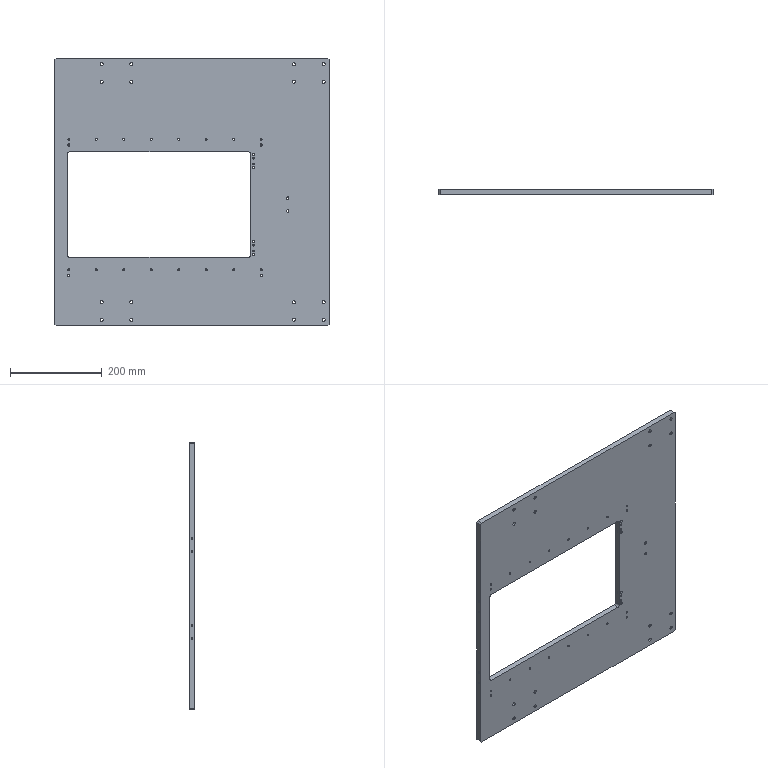Part | STEP file | PN_0008 | 1 solid | 144 faces | box 600 x 12 x 585 mm | volume 3092667 mm3 | cylinder 116 | plane 20 | cone 8 | commonest cylinder face diameters 4.2 x40 6.8 x32 10 x16 5.5 x12 4 x8 5 x8